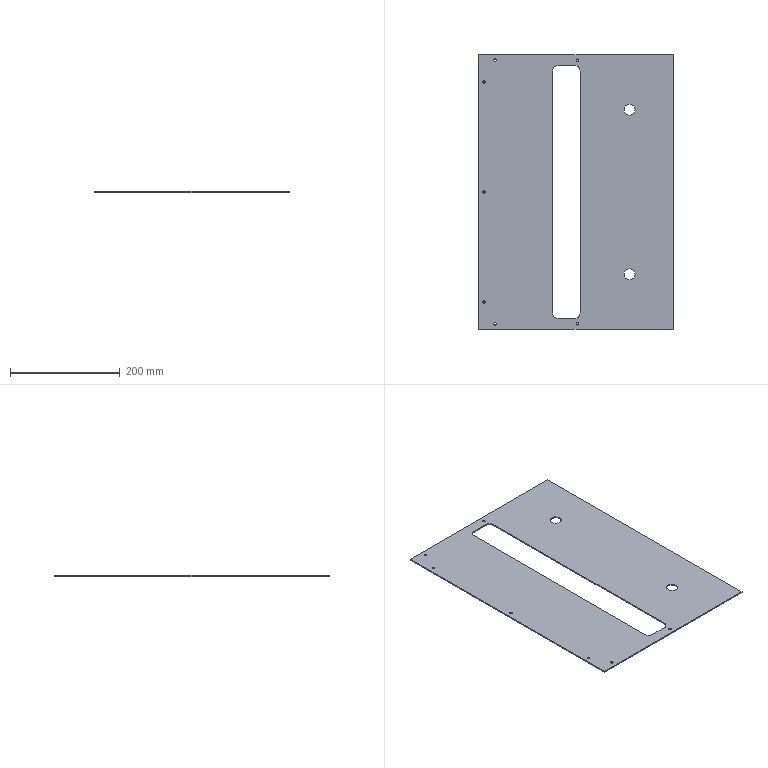Part | SolidWorks | features ICE 2, Extrusion 1, Fillet 1, HoleWzd 1 | 1 solid | 32 faces | box 355 x 500 x 2 mm | volume 307692 mm3 | cylinder 22 | plane 10 | commonest cylinder face diameters 4.5 x14 20 x8
STEP:
#1=CARTESIAN_POINT('',(87.5,150.,2.));
#2=VERTEX_POINT('',#1);
#3=CARTESIAN_POINT('',(107.5,150.,2.));
#4=VERTEX_POINT('',#3);
#5=CARTESIAN_POINT('',(97.5,150.,2.));
#6=DIRECTION('',(0.,0.,1.));
#7=DIRECTION('',(1.,0.,0.));
#8=AXIS2_PLACEMENT_3D('',#5,#6,#7);
#9=CIRCLE('',#8,10.);
#10=EDGE_CURVE('',#2,#4,#9,.T.);
#11=ORIENTED_EDGE('',*,*,#10,.T.);
#12=CARTESIAN_POINT('',(107.5,150.,0.));
#13=VERTEX_POINT('',#12);
#14=CARTESIAN_POINT('',(107.5,150.,10.));
#15=DIRECTION('',(0.,0.,-1.));
#16=VECTOR('',#15,1000.);
#17=LINE('',#14,#16);
#18=EDGE_CURVE('',#4,#13,#17,.T.);
#19=ORIENTED_EDGE('',*,*,#18,.T.);
#20=CARTESIAN_POINT('',(87.5,150.,0.));
#21=VERTEX_POINT('',#20);
#22=CARTESIAN_POINT('',(97.5,150.,0.));
#23=DIRECTION('',(0.,0.,-1.));
#24=DIRECTION('',(-1.,0.,0.));
#25=AXIS2_PLACEMENT_3D('',#22,#23,#24);
#26=CIRCLE('',#25,10.);
#27=EDGE_CURVE('',#13,#21,#26,.T.);
#28=ORIENTED_EDGE('',*,*,#27,.T.);
#29=CARTESIAN_POINT('',(87.5,150.,10.));
#30=DIRECTION('',(0.,0.,-1.));
#31=VECTOR('',#30,1000.);
#32=LINE('',#29,#31);
#33=EDGE_CURVE('',#2,#21,#32,.T.);
#34=ORIENTED_EDGE('',*,*,#33,.F.);
#35=EDGE_LOOP('',(#11,#19,#28,#34));
#36=FACE_OUTER_BOUND('',#35,.T.);
#37=CARTESIAN_POINT('',(97.5,150.,10.));
#38=DIRECTION('',(0.,0.,-1.));
#39=DIRECTION('',(-1.,0.,0.));
#40=AXIS2_PLACEMENT_3D('',#37,#38,#39);
#41=CYLINDRICAL_SURFACE('',#40,10.);
#42=ADVANCED_FACE('',(#36),#41,.F.);
#43=CARTESIAN_POINT('',(87.5,-150.,2.));
#44=VERTEX_POINT('',#43);
#45=CARTESIAN_POINT('',(107.5,-150.,2.));
#46=VERTEX_POINT('',#45);
#47=CARTESIAN_POINT('',(97.5,-150.,2.));
#48=DIRECTION('',(0.,0.,1.));
#49=DIRECTION('',(1.,0.,0.));
#50=AXIS2_PLACEMENT_3D('',#47,#48,#49);
#51=CIRCLE('',#50,10.);
#52=EDGE_CURVE('',#44,#46,#51,.T.);
#53=ORIENTED_EDGE('',*,*,#52,.T.);
#54=CARTESIAN_POINT('',(107.5,-150.,0.));
#55=VERTEX_POINT('',#54);
#56=CARTESIAN_POINT('',(107.5,-150.,10.));
#57=DIRECTION('',(0.,0.,-1.));
#58=VECTOR('',#57,1000.);
#59=LINE('',#56,#58);
#60=EDGE_CURVE('',#46,#55,#59,.T.);
#61=ORIENTED_EDGE('',*,*,#60,.T.);
#62=CARTESIAN_POINT('',(87.5,-150.,0.));
#63=VERTEX_POINT('',#62);
#64=CARTESIAN_POINT('',(97.5,-150.,0.));
#65=DIRECTION('',(0.,0.,-1.));
#66=DIRECTION('',(-1.,0.,0.));
#67=AXIS2_PLACEMENT_3D('',#64,#65,#66);
#68=CIRCLE('',#67,10.);
#69=EDGE_CURVE('',#55,#63,#68,.T.);
#70=ORIENTED_EDGE('',*,*,#69,.T.);
#71=CARTESIAN_POINT('',(87.5,-150.,10.));
#72=DIRECTION('',(0.,0.,-1.));
#73=VECTOR('',#72,1000.);
#74=LINE('',#71,#73);
#75=EDGE_CURVE('',#44,#63,#74,.T.);
#76=ORIENTED_EDGE('',*,*,#75,.F.);
#77=EDGE_LOOP('',(#53,#61,#70,#76));
#78=FACE_OUTER_BOUND('',#77,.T.);
#79=CARTESIAN_POINT('',(97.5,-150.,10.));
#80=DIRECTION('',(0.,0.,-1.));
#81=DIRECTION('',(-1.,0.,0.));
#82=AXIS2_PLACEMENT_3D('',#79,#80,#81);
#83=CYLINDRICAL_SURFACE('',#82,10.);
#84=ADVANCED_FACE('',(#78),#83,.F.);
#85=CARTESIAN_POINT('',(-169.75,0.,0.));
#86=VERTEX_POINT('',#85);
#87=CARTESIAN_POINT('',(-165.25,0.,0.));
#88=VERTEX_POINT('',#87);
#89=CARTESIAN_POINT('',(-167.5,0.,0.));
#90=DIRECTION('',(0.,0.,1.));
#91=DIRECTION('',(1.,0.,0.));
#92=AXIS2_PLACEMENT_3D('',#89,#90,#91);
#93=CIRCLE('',#92,2.25);
#94=EDGE_CURVE('',#86,#88,#93,.T.);
#95=ORIENTED_EDGE('',*,*,#94,.F.);
#96=CARTESIAN_POINT('',(-169.75,0.,2.));
#97=VERTEX_POINT('',#96);
#98=CARTESIAN_POINT('',(-169.75,0.,2.));
#99=DIRECTION('',(0.,0.,1.));
#100=VECTOR('',#99,1000.);
#101=LINE('',#98,#100);
#102=EDGE_CURVE('',#86,#97,#101,.T.);
#103=ORIENTED_EDGE('',*,*,#102,.T.);
#104=CARTESIAN_POINT('',(-165.25,0.,2.));
#105=VERTEX_POINT('',#104);
#106=CARTESIAN_POINT('',(-167.5,0.,2.));
#107=DIRECTION('',(0.,0.,1.));
#108=DIRECTION('',(1.,0.,0.));
#109=AXIS2_PLACEMENT_3D('',#106,#107,#108);
#110=CIRCLE('',#109,2.25);
#111=EDGE_CURVE('',#97,#105,#110,.T.);
#112=ORIENTED_EDGE('',*,*,#111,.T.);
#113=CARTESIAN_POINT('',(-165.25,0.,2.));
#114=DIRECTION('',(0.,0.,1.));
#115=VECTOR('',#114,1000.);
#116=LINE('',#113,#115);
#117=EDGE_CURVE('',#88,#105,#116,.T.);
#118=ORIENTED_EDGE('',*,*,#117,.F.);
#119=EDGE_LOOP('',(#95,#103,#112,#118));
#120=FACE_OUTER_BOUND('',#119,.T.);
#121=CARTESIAN_POINT('',(-167.5,0.,2.));
#122=DIRECTION('',(0.,0.,1.));
#123=DIRECTION('',(1.,0.,0.));
#124=AXIS2_PLACEMENT_3D('',#121,#122,#123);
#125=CYLINDRICAL_SURFACE('',#124,2.25);
#126=ADVANCED_FACE('',(#120),#125,.F.);
#127=CARTESIAN_POINT('',(-169.75,200.,0.));
#128=VERTEX_POINT('',#127);
#129=CARTESIAN_POINT('',(-165.25,200.,0.));
#130=VERTEX_POINT('',#129);
#131=CARTESIAN_POINT('',(-167.5,200.,0.));
#132=DIRECTION('',(0.,0.,1.));
#133=DIRECTION('',(1.,0.,0.));
#134=AXIS2_PLACEMENT_3D('',#131,#132,#133);
#135=CIRCLE('',#134,2.25);
#136=EDGE_CURVE('',#128,#130,#135,.T.);
#137=ORIENTED_EDGE('',*,*,#136,.F.);
#138=CARTESIAN_POINT('',(-169.75,200.,2.));
#139=VERTEX_POINT('',#138);
#140=CARTESIAN_POINT('',(-169.75,200.,2.));
#141=DIRECTION('',(0.,0.,1.));
#142=VECTOR('',#141,1000.);
#143=LINE('',#140,#142);
#144=EDGE_CURVE('',#128,#139,#143,.T.);
#145=ORIENTED_EDGE('',*,*,#144,.T.);
#146=CARTESIAN_POINT('',(-165.25,200.,2.));
#147=VERTEX_POINT('',#146);
#148=CARTESIAN_POINT('',(-167.5,200.,2.));
#149=DIRECTION('',(0.,0.,1.));
#150=DIRECTION('',(1.,0.,0.));
#151=AXIS2_PLACEMENT_3D('',#148,#149,#150);
#152=CIRCLE('',#151,2.25);
#153=EDGE_CURVE('',#139,#147,#152,.T.);
#154=ORIENTED_EDGE('',*,*,#153,.T.);
#155=CARTESIAN_POINT('',(-165.25,200.,2.));
#156=DIRECTION('',(0.,0.,1.));
#157=VECTOR('',#156,1000.);
#158=LINE('',#155,#157);
#159=EDGE_CURVE('',#130,#147,#158,.T.);
#160=ORIENTED_EDGE('',*,*,#159,.F.);
#161=EDGE_LOOP('',(#137,#145,#154,#160));
#162=FACE_OUTER_BOUND('',#161,.T.);
#163=CARTESIAN_POINT('',(-167.5,200.,2.));
#164=DIRECTION('',(0.,0.,1.));
#165=DIRECTION('',(1.,0.,0.));
#166=AXIS2_PLACEMENT_3D('',#163,#164,#165);
#167=CYLINDRICAL_SURFACE('',#166,2.25);
#168=ADVANCED_FACE('',(#162),#167,.F.);
#169=CARTESIAN_POINT('',(-169.75,-200.,0.));
#170=VERTEX_POINT('',#169);
#171=CARTESIAN_POINT('',(-165.25,-200.,0.));
#172=VERTEX_POINT('',#171);
#173=CARTESIAN_POINT('',(-167.5,-200.,0.));
#174=DIRECTION('',(0.,0.,1.));
#175=DIRECTION('',(1.,0.,0.));
#176=AXIS2_PLACEMENT_3D('',#173,#174,#175);
#177=CIRCLE('',#176,2.25);
#178=EDGE_CURVE('',#170,#172,#177,.T.);
#179=ORIENTED_EDGE('',*,*,#178,.F.);
#180=CARTESIAN_POINT('',(-169.75,-200.,2.));
#181=VERTEX_POINT('',#180);
#182=CARTESIAN_POINT('',(-169.75,-200.,2.));
#183=DIRECTION('',(0.,0.,1.));
#184=VECTOR('',#183,1000.);
#185=LINE('',#182,#184);
#186=EDGE_CURVE('',#170,#181,#185,.T.);
#187=ORIENTED_EDGE('',*,*,#186,.T.);
#188=CARTESIAN_POINT('',(-165.25,-200.,2.));
#189=VERTEX_POINT('',#188);
#190=CARTESIAN_POINT('',(-167.5,-200.,2.));
#191=DIRECTION('',(0.,0.,1.));
#192=DIRECTION('',(1.,0.,0.));
#193=AXIS2_PLACEMENT_3D('',#190,#191,#192);
#194=CIRCLE('',#193,2.25);
#195=EDGE_CURVE('',#181,#189,#194,.T.);
#196=ORIENTED_EDGE('',*,*,#195,.T.);
#197=CARTESIAN_POINT('',(-165.25,-200.,2.));
#198=DIRECTION('',(0.,0.,1.));
#199=VECTOR('',#198,1000.);
#200=LINE('',#197,#199);
#201=EDGE_CURVE('',#172,#189,#200,.T.);
#202=ORIENTED_EDGE('',*,*,#201,.F.);
#203=EDGE_LOOP('',(#179,#187,#196,#202));
#204=FACE_OUTER_BOUND('',#203,.T.);
#205=CARTESIAN_POINT('',(-167.5,-200.,2.));
#206=DIRECTION('',(0.,0.,1.));
#207=DIRECTION('',(1.,0.,0.));
#208=AXIS2_PLACEMENT_3D('',#205,#206,#207);
#209=CYLINDRICAL_SURFACE('',#208,2.25);
#210=ADVANCED_FACE('',(#204),#209,.F.);
#211=CARTESIAN_POINT('',(-149.75,240.,0.));
#212=VERTEX_POINT('',#211);
#213=CARTESIAN_POINT('',(-145.25,240.,0.));
#214=VERTEX_POINT('',#213);
#215=CARTESIAN_POINT('',(-147.5,240.,0.));
#216=DIRECTION('',(0.,0.,1.));
#217=DIRECTION('',(1.,0.,0.));
#218=AXIS2_PLACEMENT_3D('',#215,#216,#217);
#219=CIRCLE('',#218,2.25);
#220=EDGE_CURVE('',#212,#214,#219,.T.);
#221=ORIENTED_EDGE('',*,*,#220,.F.);
#222=CARTESIAN_POINT('',(-149.75,240.,2.));
#223=VERTEX_POINT('',#222);
#224=CARTESIAN_POINT('',(-149.75,240.,2.));
#225=DIRECTION('',(0.,0.,1.));
#226=VECTOR('',#225,1000.);
#227=LINE('',#224,#226);
#228=EDGE_CURVE('',#212,#223,#227,.T.);
#229=ORIENTED_EDGE('',*,*,#228,.T.);
#230=CARTESIAN_POINT('',(-145.25,240.,2.));
#231=VERTEX_POINT('',#230);
#232=CARTESIAN_POINT('',(-147.5,240.,2.));
#233=DIRECTION('',(0.,0.,1.));
#234=DIRECTION('',(1.,0.,0.));
#235=AXIS2_PLACEMENT_3D('',#232,#233,#234);
#236=CIRCLE('',#235,2.25);
#237=EDGE_CURVE('',#223,#231,#236,.T.);
#238=ORIENTED_EDGE('',*,*,#237,.T.);
#239=CARTESIAN_POINT('',(-145.25,240.,2.));
#240=DIRECTION('',(0.,0.,1.));
#241=VECTOR('',#240,1000.);
#242=LINE('',#239,#241);
#243=EDGE_CURVE('',#214,#231,#242,.T.);
#244=ORIENTED_EDGE('',*,*,#243,.F.);
#245=EDGE_LOOP('',(#221,#229,#238,#244));
#246=FACE_OUTER_BOUND('',#245,.T.);
#247=CARTESIAN_POINT('',(-147.5,240.,2.));
#248=DIRECTION('',(0.,0.,1.));
#249=DIRECTION('',(1.,0.,0.));
#250=AXIS2_PLACEMENT_3D('',#247,#248,#249);
#251=CYLINDRICAL_SURFACE('',#250,2.25);
#252=ADVANCED_FACE('',(#246),#251,.F.);
#253=CARTESIAN_POINT('',(0.25,240.,0.));
#254=VERTEX_POINT('',#253);
#255=CARTESIAN_POINT('',(4.75,240.,0.));
#256=VERTEX_POINT('',#255);
#257=CARTESIAN_POINT('',(2.5,240.,0.));
#258=DIRECTION('',(0.,0.,1.));
#259=DIRECTION('',(1.,0.,0.));
#260=AXIS2_PLACEMENT_3D('',#257,#258,#259);
#261=CIRCLE('',#260,2.25);
#262=EDGE_CURVE('',#254,#256,#261,.T.);
#263=ORIENTED_EDGE('',*,*,#262,.F.);
#264=CARTESIAN_POINT('',(0.25,240.,2.));
#265=VERTEX_POINT('',#264);
#266=CARTESIAN_POINT('',(0.25,240.,2.));
#267=DIRECTION('',(0.,0.,1.));
#268=VECTOR('',#267,1000.);
#269=LINE('',#266,#268);
#270=EDGE_CURVE('',#254,#265,#269,.T.);
#271=ORIENTED_EDGE('',*,*,#270,.T.);
#272=CARTESIAN_POINT('',(4.75,240.,2.));
#273=VERTEX_POINT('',#272);
#274=CARTESIAN_POINT('',(2.5,240.,2.));
#275=DIRECTION('',(0.,0.,1.));
#276=DIRECTION('',(1.,0.,0.));
#277=AXIS2_PLACEMENT_3D('',#274,#275,#276);
#278=CIRCLE('',#277,2.25);
#279=EDGE_CURVE('',#265,#273,#278,.T.);
#280=ORIENTED_EDGE('',*,*,#279,.T.);
#281=CARTESIAN_POINT('',(4.75,240.,2.));
#282=DIRECTION('',(0.,0.,1.));
#283=VECTOR('',#282,1000.);
#284=LINE('',#281,#283);
#285=EDGE_CURVE('',#256,#273,#284,.T.);
#286=ORIENTED_EDGE('',*,*,#285,.F.);
#287=EDGE_LOOP('',(#263,#271,#280,#286));
#288=FACE_OUTER_BOUND('',#287,.T.);
#289=CARTESIAN_POINT('',(2.5,240.,2.));
#290=DIRECTION('',(0.,0.,1.));
#291=DIRECTION('',(1.,0.,0.));
#292=AXIS2_PLACEMENT_3D('',#289,#290,#291);
#293=CYLINDRICAL_SURFACE('',#292,2.25);
#294=ADVANCED_FACE('',(#288),#293,.F.);
#295=CARTESIAN_POINT('',(0.25,-240.,0.));
#296=VERTEX_POINT('',#295);
#297=CARTESIAN_POINT('',(4.75,-240.,0.));
#298=VERTEX_POINT('',#297);
#299=CARTESIAN_POINT('',(2.5,-240.,0.));
#300=DIRECTION('',(0.,0.,1.));
#301=DIRECTION('',(1.,0.,0.));
#302=AXIS2_PLACEMENT_3D('',#299,#300,#301);
#303=CIRCLE('',#302,2.25);
#304=EDGE_CURVE('',#296,#298,#303,.T.);
#305=ORIENTED_EDGE('',*,*,#304,.F.);
#306=CARTESIAN_POINT('',(0.25,-240.,2.));
#307=VERTEX_POINT('',#306);
#308=CARTESIAN_POINT('',(0.25,-240.,2.));
#309=DIRECTION('',(0.,0.,1.));
#310=VECTOR('',#309,1000.);
#311=LINE('',#308,#310);
#312=EDGE_CURVE('',#296,#307,#311,.T.);
#313=ORIENTED_EDGE('',*,*,#312,.T.);
#314=CARTESIAN_POINT('',(4.75,-240.,2.));
#315=VERTEX_POINT('',#314);
#316=CARTESIAN_POINT('',(2.5,-240.,2.));
#317=DIRECTION('',(0.,0.,1.));
#318=DIRECTION('',(1.,0.,0.));
#319=AXIS2_PLACEMENT_3D('',#316,#317,#318);
#320=CIRCLE('',#319,2.25);
#321=EDGE_CURVE('',#307,#315,#320,.T.);
#322=ORIENTED_EDGE('',*,*,#321,.T.);
#323=CARTESIAN_POINT('',(4.75,-240.,2.));
#324=DIRECTION('',(0.,0.,1.));
#325=VECTOR('',#324,1000.);
#326=LINE('',#323,#325);
#327=EDGE_CURVE('',#298,#315,#326,.T.);
#328=ORIENTED_EDGE('',*,*,#327,.F.);
#329=EDGE_LOOP('',(#305,#313,#322,#328));
#330=FACE_OUTER_BOUND('',#329,.T.);
#331=CARTESIAN_POINT('',(2.5,-240.,2.));
#332=DIRECTION('',(0.,0.,1.));
#333=DIRECTION('',(1.,0.,0.));
#334=AXIS2_PLACEMENT_3D('',#331,#332,#333);
#335=CYLINDRICAL_SURFACE('',#334,2.25);
#336=ADVANCED_FACE('',(#330),#335,.F.);
#337=CARTESIAN_POINT('',(-149.75,-240.,0.));
#338=VERTEX_POINT('',#337);
#339=CARTESIAN_POINT('',(-145.25,-240.,0.));
#340=VERTEX_POINT('',#339);
#341=CARTESIAN_POINT('',(-147.5,-240.,0.));
#342=DIRECTION('',(0.,0.,1.));
#343=DIRECTION('',(1.,0.,0.));
#344=AXIS2_PLACEMENT_3D('',#341,#342,#343);
#345=CIRCLE('',#344,2.25);
#346=EDGE_CURVE('',#338,#340,#345,.T.);
#347=ORIENTED_EDGE('',*,*,#346,.F.);
#348=CARTESIAN_POINT('',(-149.75,-240.,2.));
#349=VERTEX_POINT('',#348);
#350=CARTESIAN_POINT('',(-149.75,-240.,2.));
#351=DIRECTION('',(0.,0.,1.));
#352=VECTOR('',#351,1000.);
#353=LINE('',#350,#352);
#354=EDGE_CURVE('',#338,#349,#353,.T.);
#355=ORIENTED_EDGE('',*,*,#354,.T.);
#356=CARTESIAN_POINT('',(-145.25,-240.,2.));
#357=VERTEX_POINT('',#356);
#358=CARTESIAN_POINT('',(-147.5,-240.,2.));
#359=DIRECTION('',(0.,0.,1.));
#360=DIRECTION('',(1.,0.,0.));
#361=AXIS2_PLACEMENT_3D('',#358,#359,#360);
#362=CIRCLE('',#361,2.25);
#363=EDGE_CURVE('',#349,#357,#362,.T.);
#364=ORIENTED_EDGE('',*,*,#363,.T.);
#365=CARTESIAN_POINT('',(-145.25,-240.,2.));
#366=DIRECTION('',(0.,0.,1.));
#367=VECTOR('',#366,1000.);
#368=LINE('',#365,#367);
#369=EDGE_CURVE('',#340,#357,#368,.T.);
#370=ORIENTED_EDGE('',*,*,#369,.F.);
#371=EDGE_LOOP('',(#347,#355,#364,#370));
#372=FACE_OUTER_BOUND('',#371,.T.);
#373=CARTESIAN_POINT('',(-147.5,-240.,2.));
#374=DIRECTION('',(0.,0.,1.));
#375=DIRECTION('',(1.,0.,0.));
#376=AXIS2_PLACEMENT_3D('',#373,#374,#375);
#377=CYLINDRICAL_SURFACE('',#376,2.25);
#378=ADVANCED_FACE('',(#372),#377,.F.);
#379=CARTESIAN_POINT('',(177.5,-250.,0.));
#380=VERTEX_POINT('',#379);
#381=CARTESIAN_POINT('',(177.5,250.,0.));
#382=VERTEX_POINT('',#381);
#383=CARTESIAN_POINT('',(177.5,250.,0.));
#384=DIRECTION('',(0.,1.,0.));
#385=VECTOR('',#384,1000.);
#386=LINE('',#383,#385);
#387=EDGE_CURVE('',#380,#382,#386,.T.);
#388=ORIENTED_EDGE('',*,*,#387,.T.);
#389=CARTESIAN_POINT('',(177.5,250.,2.));
#390=VERTEX_POINT('',#389);
#391=CARTESIAN_POINT('',(177.5,250.,2.));
#392=DIRECTION('',(0.,0.,-1.));
#393=VECTOR('',#392,1000.);
#394=LINE('',#391,#393);
#395=EDGE_CURVE('',#390,#382,#394,.T.);
#396=ORIENTED_EDGE('',*,*,#395,.F.);
#397=CARTESIAN_POINT('',(177.5,-250.,2.));
#398=VERTEX_POINT('',#397);
#399=CARTESIAN_POINT('',(177.5,250.,2.));
#400=DIRECTION('',(0.,1.,0.));
#401=VECTOR('',#400,1000.);
#402=LINE('',#399,#401);
#403=EDGE_CURVE('',#398,#390,#402,.T.);
#404=ORIENTED_EDGE('',*,*,#403,.F.);
#405=CARTESIAN_POINT('',(177.5,-250.,2.));
#406=DIRECTION('',(0.,0.,-1.));
#407=VECTOR('',#406,1000.);
#408=LINE('',#405,#407);
#409=EDGE_CURVE('',#398,#380,#408,.T.);
#410=ORIENTED_EDGE('',*,*,#409,.T.);
#411=EDGE_LOOP('',(#388,#396,#404,#410));
#412=FACE_OUTER_BOUND('',#411,.T.);
#413=CARTESIAN_POINT('',(177.5,250.,2.));
#414=DIRECTION('',(-1.,0.,0.));
#415=DIRECTION('',(0.,0.,1.));
#416=AXIS2_PLACEMENT_3D('',#413,#414,#415);
#417=PLANE('',#416);
#418=ADVANCED_FACE('',(#412),#417,.F.);
#419=CARTESIAN_POINT('',(-177.5,250.,0.));
#420=VERTEX_POINT('',#419);
#421=CARTESIAN_POINT('',(-177.5,250.,0.));
#422=DIRECTION('',(-1.,0.,0.));
#423=VECTOR('',#422,1000.);
#424=LINE('',#421,#423);
#425=EDGE_CURVE('',#382,#420,#424,.T.);
#426=ORIENTED_EDGE('',*,*,#425,.T.);
#427=CARTESIAN_POINT('',(-177.5,250.,2.));
#428=VERTEX_POINT('',#427);
#429=CARTESIAN_POINT('',(-177.5,250.,2.));
#430=DIRECTION('',(0.,0.,-1.));
#431=VECTOR('',#430,1000.);
#432=LINE('',#429,#431);
#433=EDGE_CURVE('',#428,#420,#432,.T.);
#434=ORIENTED_EDGE('',*,*,#433,.F.);
#435=CARTESIAN_POINT('',(-177.5,250.,2.));
#436=DIRECTION('',(-1.,0.,0.));
#437=VECTOR('',#436,1000.);
#438=LINE('',#435,#437);
#439=EDGE_CURVE('',#390,#428,#438,.T.);
#440=ORIENTED_EDGE('',*,*,#439,.F.);
#441=ORIENTED_EDGE('',*,*,#395,.T.);
#442=EDGE_LOOP('',(#426,#434,#440,#441));
#443=FACE_OUTER_BOUND('',#442,.T.);
#444=CARTESIAN_POINT('',(-177.5,250.,2.));
#445=DIRECTION('',(0.,-1.,0.));
#446=DIRECTION('',(0.,0.,-1.));
#447=AXIS2_PLACEMENT_3D('',#444,#445,#446);
#448=PLANE('',#447);
#449=ADVANCED_FACE('',(#443),#448,.F.);
#450=CARTESIAN_POINT('',(-177.5,-250.,0.));
#451=VERTEX_POINT('',#450);
#452=CARTESIAN_POINT('',(-177.5,250.,0.));
#453=DIRECTION('',(0.,-1.,0.));
#454=VECTOR('',#453,1000.);
#455=LINE('',#452,#454);
#456=EDGE_CURVE('',#420,#451,#455,.T.);
#457=ORIENTED_EDGE('',*,*,#456,.T.);
#458=CARTESIAN_POINT('',(-177.5,-250.,2.));
#459=VERTEX_POINT('',#458);
#460=CARTESIAN_POINT('',(-177.5,-250.,2.));
#461=DIRECTION('',(0.,0.,-1.));
#462=VECTOR('',#461,1000.);
#463=LINE('',#460,#462);
#464=EDGE_CURVE('',#459,#451,#463,.T.);
#465=ORIENTED_EDGE('',*,*,#464,.F.);
#466=CARTESIAN_POINT('',(-177.5,250.,2.));
#467=DIRECTION('',(0.,-1.,0.));
#468=VECTOR('',#467,1000.);
#469=LINE('',#466,#468);
#470=EDGE_CURVE('',#428,#459,#469,.T.);
#471=ORIENTED_EDGE('',*,*,#470,.F.);
#472=ORIENTED_EDGE('',*,*,#433,.T.);
#473=EDGE_LOOP('',(#457,#465,#471,#472));
#474=FACE_OUTER_BOUND('',#473,.T.);
#475=CARTESIAN_POINT('',(-177.5,250.,2.));
#476=DIRECTION('',(1.,0.,0.));
#477=DIRECTION('',(0.,0.,-1.));
#478=AXIS2_PLACEMENT_3D('',#475,#476,#477);
#479=PLANE('',#478);
#480=ADVANCED_FACE('',(#474),#479,.F.);
#481=CARTESIAN_POINT('',(-177.5,-250.,0.));
#482=DIRECTION('',(1.,0.,0.));
#483=VECTOR('',#482,1000.);
#484=LINE('',#481,#483);
#485=EDGE_CURVE('',#451,#380,#484,.T.);
#486=ORIENTED_EDGE('',*,*,#485,.T.);
#487=ORIENTED_EDGE('',*,*,#409,.F.);
#488=CARTESIAN_POINT('',(-177.5,-250.,2.));
#489=DIRECTION('',(1.,0.,0.));
#490=VECTOR('',#489,1000.);
#491=LINE('',#488,#490);
#492=EDGE_CURVE('',#459,#398,#491,.T.);
#493=ORIENTED_EDGE('',*,*,#492,.F.);
#494=ORIENTED_EDGE('',*,*,#464,.T.);
#495=EDGE_LOOP('',(#486,#487,#493,#494));
#496=FACE_OUTER_BOUND('',#495,.T.);
#497=CARTESIAN_POINT('',(-177.5,-250.,2.));
#498=DIRECTION('',(0.,1.,0.));
#499=DIRECTION('',(0.,0.,1.));
#500=AXIS2_PLACEMENT_3D('',#497,#498,#499);
#501=PLANE('',#500);
#502=ADVANCED_FACE('',(#496),#501,.F.);
#503=ORIENTED_EDGE('',*,*,#10,.F.);
#504=CARTESIAN_POINT('',(97.5,150.,2.));
#505=DIRECTION('',(0.,0.,1.));
#506=DIRECTION('',(1.,0.,0.));
#507=AXIS2_PLACEMENT_3D('',#504,#505,#506);
#508=CIRCLE('',#507,10.);
#509=EDGE_CURVE('',#4,#2,#508,.T.);
#510=ORIENTED_EDGE('',*,*,#509,.F.);
#511=EDGE_LOOP('',(#503,#510));
#512=FACE_BOUND('',#511,.T.);
#513=ORIENTED_EDGE('',*,*,#52,.F.);
#514=CARTESIAN_POINT('',(97.5,-150.,2.));
#515=DIRECTION('',(0.,0.,1.));
#516=DIRECTION('',(1.,0.,0.));
#517=AXIS2_PLACEMENT_3D('',#514,#515,#516);
#518=CIRCLE('',#517,10.);
#519=EDGE_CURVE('',#46,#44,#518,.T.);
#520=ORIENTED_EDGE('',*,*,#519,.F.);
#521=EDGE_LOOP('',(#513,#520));
#522=FACE_BOUND('',#521,.T.);
#523=CARTESIAN_POINT('',(-42.5,220.,2.));
#524=VERTEX_POINT('',#523);
#525=CARTESIAN_POINT('',(-42.5,-220.,2.));
#526=VERTEX_POINT('',#525);
#527=CARTESIAN_POINT('',(-42.5,0.,2.));
#528=DIRECTION('',(0.,-1.,0.));
#529=VECTOR('',#528,1000.);
#530=LINE('',#527,#529);
#531=EDGE_CURVE('',#524,#526,#530,.T.);
#532=ORIENTED_EDGE('',*,*,#531,.F.);
#533=CARTESIAN_POINT('',(-32.5,230.,2.));
#534=VERTEX_POINT('',#533);
#535=CARTESIAN_POINT('',(-32.5,220.,2.));
#536=DIRECTION('',(0.,0.,-1.));
#537=DIRECTION('',(1.,0.,0.));
#538=AXIS2_PLACEMENT_3D('',#535,#536,#537);
#539=CIRCLE('',#538,10.);
#540=EDGE_CURVE('',#524,#534,#539,.T.);
#541=ORIENTED_EDGE('',*,*,#540,.T.);
#542=CARTESIAN_POINT('',(-2.5,230.,2.));
#543=VERTEX_POINT('',#542);
#544=CARTESIAN_POINT('',(0.,230.,2.));
#545=DIRECTION('',(-1.,0.,0.));
#546=VECTOR('',#545,1000.);
#547=LINE('',#544,#546);
#548=EDGE_CURVE('',#543,#534,#547,.T.);
#549=ORIENTED_EDGE('',*,*,#548,.F.);
#550=CARTESIAN_POINT('',(7.5,220.,2.));
#551=VERTEX_POINT('',#550);
#552=CARTESIAN_POINT('',(-2.5,220.,2.));
#553=DIRECTION('',(0.,0.,-1.));
#554=DIRECTION('',(1.,0.,0.));
#555=AXIS2_PLACEMENT_3D('',#552,#553,#554);
#556=CIRCLE('',#555,10.);
#557=EDGE_CURVE('',#543,#551,#556,.T.);
#558=ORIENTED_EDGE('',*,*,#557,.T.);
#559=CARTESIAN_POINT('',(7.5,-220.,2.));
#560=VERTEX_POINT('',#559);
#561=CARTESIAN_POINT('',(7.5,0.,2.));
#562=DIRECTION('',(0.,1.,0.));
#563=VECTOR('',#562,1000.);
#564=LINE('',#561,#563);
#565=EDGE_CURVE('',#560,#551,#564,.T.);
#566=ORIENTED_EDGE('',*,*,#565,.F.);
#567=CARTESIAN_POINT('',(-2.5,-230.,2.));
#568=VERTEX_POINT('',#567);
#569=CARTESIAN_POINT('',(-2.5,-220.,2.));
#570=DIRECTION('',(0.,0.,-1.));
#571=DIRECTION('',(1.,0.,0.));
#572=AXIS2_PLACEMENT_3D('',#569,#570,#571);
#573=CIRCLE('',#572,10.);
#574=EDGE_CURVE('',#560,#568,#573,.T.);
#575=ORIENTED_EDGE('',*,*,#574,.T.);
#576=CARTESIAN_POINT('',(-32.5,-230.,2.));
#577=VERTEX_POINT('',#576);
#578=CARTESIAN_POINT('',(0.,-230.,2.));
#579=DIRECTION('',(1.,0.,0.));
#580=VECTOR('',#579,1000.);
#581=LINE('',#578,#580);
#582=EDGE_CURVE('',#577,#568,#581,.T.);
#583=ORIENTED_EDGE('',*,*,#582,.F.);
#584=CARTESIAN_POINT('',(-32.5,-220.,2.));
#585=DIRECTION('',(0.,0.,-1.));
#586=DIRECTION('',(1.,0.,0.));
#587=AXIS2_PLACEMENT_3D('',#584,#585,#586);
#588=CIRCLE('',#587,10.);
#589=EDGE_CURVE('',#577,#526,#588,.T.);
#590=ORIENTED_EDGE('',*,*,#589,.T.);
#591=EDGE_LOOP('',(#532,#541,#549,#558,#566,#575,#583,#590));
#592=FACE_BOUND('',#591,.T.);
#593=CARTESIAN_POINT('',(-167.5,0.,2.));
#594=DIRECTION('',(0.,0.,1.));
#595=DIRECTION('',(1.,0.,0.));
#596=AXIS2_PLACEMENT_3D('',#593,#594,#595);
#597=CIRCLE('',#596,2.25);
#598=EDGE_CURVE('',#105,#97,#597,.T.);
#599=ORIENTED_EDGE('',*,*,#598,.F.);
#600=ORIENTED_EDGE('',*,*,#111,.F.);
#601=EDGE_LOOP('',(#599,#600));
#602=FACE_BOUND('',#601,.T.);
#603=CARTESIAN_POINT('',(-167.5,200.,2.));
#604=DIRECTION('',(0.,0.,1.));
#605=DIRECTION('',(1.,0.,0.));
#606=AXIS2_PLACEMENT_3D('',#603,#604,#605);
#607=CIRCLE('',#606,2.25);
#608=EDGE_CURVE('',#147,#139,#607,.T.);
#609=ORIENTED_EDGE('',*,*,#608,.F.);
#610=ORIENTED_EDGE('',*,*,#153,.F.);
#611=EDGE_LOOP('',(#609,#610));
#612=FACE_BOUND('',#611,.T.);
#613=CARTESIAN_POINT('',(-167.5,-200.,2.));
#614=DIRECTION('',(0.,0.,1.));
#615=DIRECTION('',(1.,0.,0.));
#616=AXIS2_PLACEMENT_3D('',#613,#614,#615);
#617=CIRCLE('',#616,2.25);
#618=EDGE_CURVE('',#189,#181,#617,.T.);
#619=ORIENTED_EDGE('',*,*,#618,.F.);
#620=ORIENTED_EDGE('',*,*,#195,.F.);
#621=EDGE_LOOP('',(#619,#620));
#622=FACE_BOUND('',#621,.T.);
#623=CARTESIAN_POINT('',(-147.5,240.,2.));
#624=DIRECTION('',(0.,0.,1.));
#625=DIRECTION('',(1.,0.,0.));
#626=AXIS2_PLACEMENT_3D('',#623,#624,#625);
#627=CIRCLE('',#626,2.25);
#628=EDGE_CURVE('',#231,#223,#627,.T.);
#629=ORIENTED_EDGE('',*,*,#628,.F.);
#630=ORIENTED_EDGE('',*,*,#237,.F.);
#631=EDGE_LOOP('',(#629,#630));
#632=FACE_BOUND('',#631,.T.);
#633=CARTESIAN_POINT('',(2.5,240.,2.));
#634=DIRECTION('',(0.,0.,1.));
#635=DIRECTION('',(1.,0.,0.));
#636=AXIS2_PLACEMENT_3D('',#633,#634,#635);
#637=CIRCLE('',#636,2.25);
#638=EDGE_CURVE('',#273,#265,#637,.T.);
#639=ORIENTED_EDGE('',*,*,#638,.F.);
#640=ORIENTED_EDGE('',*,*,#279,.F.);
#641=EDGE_LOOP('',(#639,#640));
#642=FACE_BOUND('',#641,.T.);
#643=CARTESIAN_POINT('',(2.5,-240.,2.));
#644=DIRECTION('',(0.,0.,1.));
#645=DIRECTION('',(1.,0.,0.));
#646=AXIS2_PLACEMENT_3D('',#643,#644,#645);
#647=CIRCLE('',#646,2.25);
#648=EDGE_CURVE('',#315,#307,#647,.T.);
#649=ORIENTED_EDGE('',*,*,#648,.F.);
#650=ORIENTED_EDGE('',*,*,#321,.F.);
#651=EDGE_LOOP('',(#649,#650));
#652=FACE_BOUND('',#651,.T.);
#653=CARTESIAN_POINT('',(-147.5,-240.,2.));
#654=DIRECTION('',(0.,0.,1.));
#655=DIRECTION('',(1.,0.,0.));
#656=AXIS2_PLACEMENT_3D('',#653,#654,#655);
#657=CIRCLE('',#656,2.25);
#658=EDGE_CURVE('',#357,#349,#657,.T.);
#659=ORIENTED_EDGE('',*,*,#658,.F.);
#660=ORIENTED_EDGE('',*,*,#363,.F.);
#661=EDGE_LOOP('',(#659,#660));
#662=FACE_BOUND('',#661,.T.);
#663=ORIENTED_EDGE('',*,*,#403,.T.);
#664=ORIENTED_EDGE('',*,*,#439,.T.);
#665=ORIENTED_EDGE('',*,*,#470,.T.);
#666=ORIENTED_EDGE('',*,*,#492,.T.);
#667=EDGE_LOOP('',(#663,#664,#665,#666));
#668=FACE_OUTER_BOUND('',#667,.T.);
#669=CARTESIAN_POINT('',(0.,0.,2.));
#670=DIRECTION('',(0.,0.,1.));
#671=DIRECTION('',(1.,0.,0.));
#672=AXIS2_PLACEMENT_3D('',#669,#670,#671);
#673=PLANE('',#672);
#674=ADVANCED_FACE('',(#512,#522,#592,#602,#612,#622,#632,#642,#652,#662,#668),#673,.T.);
#675=CARTESIAN_POINT('',(97.5,150.,0.));
#676=DIRECTION('',(0.,0.,-1.));
#677=DIRECTION('',(-1.,0.,0.));
#678=AXIS2_PLACEMENT_3D('',#675,#676,#677);
#679=CIRCLE('',#678,10.);
#680=EDGE_CURVE('',#21,#13,#679,.T.);
#681=ORIENTED_EDGE('',*,*,#680,.F.);
#682=ORIENTED_EDGE('',*,*,#27,.F.);
#683=EDGE_LOOP('',(#681,#682));
#684=FACE_BOUND('',#683,.T.);
#685=CARTESIAN_POINT('',(97.5,-150.,0.));
#686=DIRECTION('',(0.,0.,-1.));
#687=DIRECTION('',(-1.,0.,0.));
#688=AXIS2_PLACEMENT_3D('',#685,#686,#687);
#689=CIRCLE('',#688,10.);
#690=EDGE_CURVE('',#63,#55,#689,.T.);
#691=ORIENTED_EDGE('',*,*,#690,.F.);
#692=ORIENTED_EDGE('',*,*,#69,.F.);
#693=EDGE_LOOP('',(#691,#692));
#694=FACE_BOUND('',#693,.T.);
#695=CARTESIAN_POINT('',(-32.5,230.,0.));
#696=VERTEX_POINT('',#695);
#697=CARTESIAN_POINT('',(-2.5,230.,0.));
#698=VERTEX_POINT('',#697);
#699=CARTESIAN_POINT('',(7.5,230.,0.));
#700=DIRECTION('',(1.,0.,0.));
#701=VECTOR('',#700,1000.);
#702=LINE('',#699,#701);
#703=EDGE_CURVE('',#696,#698,#702,.T.);
#704=ORIENTED_EDGE('',*,*,#703,.F.);
#705=CARTESIAN_POINT('',(-42.5,220.,0.));
#706=VERTEX_POINT('',#705);
#707=CARTESIAN_POINT('',(-32.5,220.,0.));
#708=DIRECTION('',(0.,0.,1.));
#709=DIRECTION('',(1.,0.,0.));
#710=AXIS2_PLACEMENT_3D('',#707,#708,#709);
#711=CIRCLE('',#710,10.);
#712=EDGE_CURVE('',#696,#706,#711,.T.);
#713=ORIENTED_EDGE('',*,*,#712,.T.);
#714=CARTESIAN_POINT('',(-42.5,-220.,0.));
#715=VERTEX_POINT('',#714);
#716=CARTESIAN_POINT('',(-42.5,-230.,0.));
#717=DIRECTION('',(0.,1.,0.));
#718=VECTOR('',#717,1000.);
#719=LINE('',#716,#718);
#720=EDGE_CURVE('',#715,#706,#719,.T.);
#721=ORIENTED_EDGE('',*,*,#720,.F.);
#722=CARTESIAN_POINT('',(-32.5,-230.,0.));
#723=VERTEX_POINT('',#722);
#724=CARTESIAN_POINT('',(-32.5,-220.,0.));
#725=DIRECTION('',(0.,0.,1.));
#726=DIRECTION('',(1.,0.,0.));
#727=AXIS2_PLACEMENT_3D('',#724,#725,#726);
#728=CIRCLE('',#727,10.);
#729=EDGE_CURVE('',#715,#723,#728,.T.);
#730=ORIENTED_EDGE('',*,*,#729,.T.);
#731=CARTESIAN_POINT('',(-2.5,-230.,0.));
#732=VERTEX_POINT('',#731);
#733=CARTESIAN_POINT('',(7.5,-230.,0.));
#734=DIRECTION('',(-1.,0.,0.));
#735=VECTOR('',#734,1000.);
#736=LINE('',#733,#735);
#737=EDGE_CURVE('',#732,#723,#736,.T.);
#738=ORIENTED_EDGE('',*,*,#737,.F.);
#739=CARTESIAN_POINT('',(7.5,-220.,0.));
#740=VERTEX_POINT('',#739);
#741=CARTESIAN_POINT('',(-2.5,-220.,0.));
#742=DIRECTION('',(0.,0.,1.));
#743=DIRECTION('',(1.,0.,0.));
#744=AXIS2_PLACEMENT_3D('',#741,#742,#743);
#745=CIRCLE('',#744,10.);
#746=EDGE_CURVE('',#732,#740,#745,.T.);
#747=ORIENTED_EDGE('',*,*,#746,.T.);
#748=CARTESIAN_POINT('',(7.5,220.,0.));
#749=VERTEX_POINT('',#748);
#750=CARTESIAN_POINT('',(7.5,-230.,0.));
#751=DIRECTION('',(0.,-1.,0.));
#752=VECTOR('',#751,1000.);
#753=LINE('',#750,#752);
#754=EDGE_CURVE('',#749,#740,#753,.T.);
#755=ORIENTED_EDGE('',*,*,#754,.F.);
#756=CARTESIAN_POINT('',(-2.5,220.,0.));
#757=DIRECTION('',(0.,0.,1.));
#758=DIRECTION('',(1.,0.,0.));
#759=AXIS2_PLACEMENT_3D('',#756,#757,#758);
#760=CIRCLE('',#759,10.);
#761=EDGE_CURVE('',#749,#698,#760,.T.);
#762=ORIENTED_EDGE('',*,*,#761,.T.);
#763=EDGE_LOOP('',(#704,#713,#721,#730,#738,#747,#755,#762));
#764=FACE_BOUND('',#763,.T.);
#765=CARTESIAN_POINT('',(-167.5,0.,0.));
#766=DIRECTION('',(0.,0.,1.));
#767=DIRECTION('',(1.,0.,0.));
#768=AXIS2_PLACEMENT_3D('',#765,#766,#767);
#769=CIRCLE('',#768,2.25);
#770=EDGE_CURVE('',#88,#86,#769,.T.);
#771=ORIENTED_EDGE('',*,*,#770,.T.);
#772=ORIENTED_EDGE('',*,*,#94,.T.);
#773=EDGE_LOOP('',(#771,#772));
#774=FACE_BOUND('',#773,.T.);
#775=CARTESIAN_POINT('',(-167.5,200.,0.));
#776=DIRECTION('',(0.,0.,1.));
#777=DIRECTION('',(1.,0.,0.));
#778=AXIS2_PLACEMENT_3D('',#775,#776,#777);
#779=CIRCLE('',#778,2.25);
#780=EDGE_CURVE('',#130,#128,#779,.T.);
#781=ORIENTED_EDGE('',*,*,#780,.T.);
#782=ORIENTED_EDGE('',*,*,#136,.T.);
#783=EDGE_LOOP('',(#781,#782));
#784=FACE_BOUND('',#783,.T.);
#785=CARTESIAN_POINT('',(-167.5,-200.,0.));
#786=DIRECTION('',(0.,0.,1.));
#787=DIRECTION('',(1.,0.,0.));
#788=AXIS2_PLACEMENT_3D('',#785,#786,#787);
#789=CIRCLE('',#788,2.25);
#790=EDGE_CURVE('',#172,#170,#789,.T.);
#791=ORIENTED_EDGE('',*,*,#790,.T.);
#792=ORIENTED_EDGE('',*,*,#178,.T.);
#793=EDGE_LOOP('',(#791,#792));
#794=FACE_BOUND('',#793,.T.);
#795=CARTESIAN_POINT('',(-147.5,240.,0.));
#796=DIRECTION('',(0.,0.,1.));
#797=DIRECTION('',(1.,0.,0.));
#798=AXIS2_PLACEMENT_3D('',#795,#796,#797);
#799=CIRCLE('',#798,2.25);
#800=EDGE_CURVE('',#214,#212,#799,.T.);
#801=ORIENTED_EDGE('',*,*,#800,.T.);
#802=ORIENTED_EDGE('',*,*,#220,.T.);
#803=EDGE_LOOP('',(#801,#802));
#804=FACE_BOUND('',#803,.T.);
#805=CARTESIAN_POINT('',(2.5,240.,0.));
#806=DIRECTION('',(0.,0.,1.));
#807=DIRECTION('',(1.,0.,0.));
#808=AXIS2_PLACEMENT_3D('',#805,#806,#807);
#809=CIRCLE('',#808,2.25);
#810=EDGE_CURVE('',#256,#254,#809,.T.);
#811=ORIENTED_EDGE('',*,*,#810,.T.);
#812=ORIENTED_EDGE('',*,*,#262,.T.);
#813=EDGE_LOOP('',(#811,#812));
#814=FACE_BOUND('',#813,.T.);
#815=CARTESIAN_POINT('',(2.5,-240.,0.));
#816=DIRECTION('',(0.,0.,1.));
#817=DIRECTION('',(1.,0.,0.));
#818=AXIS2_PLACEMENT_3D('',#815,#816,#817);
#819=CIRCLE('',#818,2.25);
#820=EDGE_CURVE('',#298,#296,#819,.T.);
#821=ORIENTED_EDGE('',*,*,#820,.T.);
#822=ORIENTED_EDGE('',*,*,#304,.T.);
#823=EDGE_LOOP('',(#821,#822));
#824=FACE_BOUND('',#823,.T.);
#825=CARTESIAN_POINT('',(-147.5,-240.,0.));
#826=DIRECTION('',(0.,0.,1.));
#827=DIRECTION('',(1.,0.,0.));
#828=AXIS2_PLACEMENT_3D('',#825,#826,#827);
#829=CIRCLE('',#828,2.25);
#830=EDGE_CURVE('',#340,#338,#829,.T.);
#831=ORIENTED_EDGE('',*,*,#830,.T.);
#832=ORIENTED_EDGE('',*,*,#346,.T.);
#833=EDGE_LOOP('',(#831,#832));
#834=FACE_BOUND('',#833,.T.);
#835=ORIENTED_EDGE('',*,*,#387,.F.);
#836=ORIENTED_EDGE('',*,*,#485,.F.);
#837=ORIENTED_EDGE('',*,*,#456,.F.);
#838=ORIENTED_EDGE('',*,*,#425,.F.);
#839=EDGE_LOOP('',(#835,#836,#837,#838));
#840=FACE_OUTER_BOUND('',#839,.T.);
#841=CARTESIAN_POINT('',(0.,0.,0.));
#842=DIRECTION('',(0.,0.,1.));
#843=DIRECTION('',(1.,0.,0.));
#844=AXIS2_PLACEMENT_3D('',#841,#842,#843);
#845=PLANE('',#844);
#846=ADVANCED_FACE('',(#684,#694,#764,#774,#784,#794,#804,#814,#824,#834,#840),#845,.F.);
#847=ORIENTED_EDGE('',*,*,#354,.F.);
#848=ORIENTED_EDGE('',*,*,#830,.F.);
#849=ORIENTED_EDGE('',*,*,#369,.T.);
#850=ORIENTED_EDGE('',*,*,#658,.T.);
#851=EDGE_LOOP('',(#847,#848,#849,#850));
#852=FACE_OUTER_BOUND('',#851,.T.);
#853=CARTESIAN_POINT('',(-147.5,-240.,2.));
#854=DIRECTION('',(0.,0.,1.));
#855=DIRECTION('',(1.,0.,0.));
#856=AXIS2_PLACEMENT_3D('',#853,#854,#855);
#857=CYLINDRICAL_SURFACE('',#856,2.25);
#858=ADVANCED_FACE('',(#852),#857,.F.);
#859=ORIENTED_EDGE('',*,*,#312,.F.);
#860=ORIENTED_EDGE('',*,*,#820,.F.);
#861=ORIENTED_EDGE('',*,*,#327,.T.);
#862=ORIENTED_EDGE('',*,*,#648,.T.);
#863=EDGE_LOOP('',(#859,#860,#861,#862));
#864=FACE_OUTER_BOUND('',#863,.T.);
#865=CARTESIAN_POINT('',(2.5,-240.,2.));
#866=DIRECTION('',(0.,0.,1.));
#867=DIRECTION('',(1.,0.,0.));
#868=AXIS2_PLACEMENT_3D('',#865,#866,#867);
#869=CYLINDRICAL_SURFACE('',#868,2.25);
#870=ADVANCED_FACE('',(#864),#869,.F.);
#871=ORIENTED_EDGE('',*,*,#270,.F.);
#872=ORIENTED_EDGE('',*,*,#810,.F.);
#873=ORIENTED_EDGE('',*,*,#285,.T.);
#874=ORIENTED_EDGE('',*,*,#638,.T.);
#875=EDGE_LOOP('',(#871,#872,#873,#874));
#876=FACE_OUTER_BOUND('',#875,.T.);
#877=CARTESIAN_POINT('',(2.5,240.,2.));
#878=DIRECTION('',(0.,0.,1.));
#879=DIRECTION('',(1.,0.,0.));
#880=AXIS2_PLACEMENT_3D('',#877,#878,#879);
#881=CYLINDRICAL_SURFACE('',#880,2.25);
#882=ADVANCED_FACE('',(#876),#881,.F.);
#883=ORIENTED_EDGE('',*,*,#228,.F.);
#884=ORIENTED_EDGE('',*,*,#800,.F.);
#885=ORIENTED_EDGE('',*,*,#243,.T.);
#886=ORIENTED_EDGE('',*,*,#628,.T.);
#887=EDGE_LOOP('',(#883,#884,#885,#886));
#888=FACE_OUTER_BOUND('',#887,.T.);
#889=CARTESIAN_POINT('',(-147.5,240.,2.));
#890=DIRECTION('',(0.,0.,1.));
#891=DIRECTION('',(1.,0.,0.));
#892=AXIS2_PLACEMENT_3D('',#889,#890,#891);
#893=CYLINDRICAL_SURFACE('',#892,2.25);
#894=ADVANCED_FACE('',(#888),#893,.F.);
#895=ORIENTED_EDGE('',*,*,#186,.F.);
#896=ORIENTED_EDGE('',*,*,#790,.F.);
#897=ORIENTED_EDGE('',*,*,#201,.T.);
#898=ORIENTED_EDGE('',*,*,#618,.T.);
#899=EDGE_LOOP('',(#895,#896,#897,#898));
#900=FACE_OUTER_BOUND('',#899,.T.);
#901=CARTESIAN_POINT('',(-167.5,-200.,2.));
#902=DIRECTION('',(0.,0.,1.));
#903=DIRECTION('',(1.,0.,0.));
#904=AXIS2_PLACEMENT_3D('',#901,#902,#903);
#905=CYLINDRICAL_SURFACE('',#904,2.25);
#906=ADVANCED_FACE('',(#900),#905,.F.);
#907=ORIENTED_EDGE('',*,*,#144,.F.);
#908=ORIENTED_EDGE('',*,*,#780,.F.);
#909=ORIENTED_EDGE('',*,*,#159,.T.);
#910=ORIENTED_EDGE('',*,*,#608,.T.);
#911=EDGE_LOOP('',(#907,#908,#909,#910));
#912=FACE_OUTER_BOUND('',#911,.T.);
#913=CARTESIAN_POINT('',(-167.5,200.,2.));
#914=DIRECTION('',(0.,0.,1.));
#915=DIRECTION('',(1.,0.,0.));
#916=AXIS2_PLACEMENT_3D('',#913,#914,#915);
#917=CYLINDRICAL_SURFACE('',#916,2.25);
#918=ADVANCED_FACE('',(#912),#917,.F.);
#919=ORIENTED_EDGE('',*,*,#102,.F.);
#920=ORIENTED_EDGE('',*,*,#770,.F.);
#921=ORIENTED_EDGE('',*,*,#117,.T.);
#922=ORIENTED_EDGE('',*,*,#598,.T.);
#923=EDGE_LOOP('',(#919,#920,#921,#922));
#924=FACE_OUTER_BOUND('',#923,.T.);
#925=CARTESIAN_POINT('',(-167.5,0.,2.));
#926=DIRECTION('',(0.,0.,1.));
#927=DIRECTION('',(1.,0.,0.));
#928=AXIS2_PLACEMENT_3D('',#925,#926,#927);
#929=CYLINDRICAL_SURFACE('',#928,2.25);
#930=ADVANCED_FACE('',(#924),#929,.F.);
#931=ORIENTED_EDGE('',*,*,#531,.T.);
#932=CARTESIAN_POINT('',(-42.5,-220.,0.));
#933=DIRECTION('',(0.,0.,-1.));
#934=VECTOR('',#933,1000.);
#935=LINE('',#932,#934);
#936=EDGE_CURVE('',#526,#715,#935,.T.);
#937=ORIENTED_EDGE('',*,*,#936,.T.);
#938=ORIENTED_EDGE('',*,*,#720,.T.);
#939=CARTESIAN_POINT('',(-42.5,220.,2.));
#940=DIRECTION('',(0.,0.,1.));
#941=VECTOR('',#940,1000.);
#942=LINE('',#939,#941);
#943=EDGE_CURVE('',#706,#524,#942,.T.);
#944=ORIENTED_EDGE('',*,*,#943,.T.);
#945=EDGE_LOOP('',(#931,#937,#938,#944));
#946=FACE_OUTER_BOUND('',#945,.T.);
#947=CARTESIAN_POINT('',(-42.5,-230.,10.));
#948=DIRECTION('',(-1.,0.,0.));
#949=DIRECTION('',(0.,0.,1.));
#950=AXIS2_PLACEMENT_3D('',#947,#948,#949);
#951=PLANE('',#950);
#952=ADVANCED_FACE('',(#946),#951,.F.);
#953=ORIENTED_EDGE('',*,*,#737,.T.);
#954=CARTESIAN_POINT('',(-32.5,-230.,2.));
#955=DIRECTION('',(0.,0.,1.));
#956=VECTOR('',#955,1000.);
#957=LINE('',#954,#956);
#958=EDGE_CURVE('',#723,#577,#957,.T.);
#959=ORIENTED_EDGE('',*,*,#958,.T.);
#960=ORIENTED_EDGE('',*,*,#582,.T.);
#961=CARTESIAN_POINT('',(-2.5,-230.,0.));
#962=DIRECTION('',(0.,0.,-1.));
#963=VECTOR('',#962,1000.);
#964=LINE('',#961,#963);
#965=EDGE_CURVE('',#568,#732,#964,.T.);
#966=ORIENTED_EDGE('',*,*,#965,.T.);
#967=EDGE_LOOP('',(#953,#959,#960,#966));
#968=FACE_OUTER_BOUND('',#967,.T.);
#969=CARTESIAN_POINT('',(7.5,-230.,10.));
#970=DIRECTION('',(0.,-1.,0.));
#971=DIRECTION('',(0.,0.,-1.));
#972=AXIS2_PLACEMENT_3D('',#969,#970,#971);
#973=PLANE('',#972);
#974=ADVANCED_FACE('',(#968),#973,.F.);
#975=ORIENTED_EDGE('',*,*,#754,.T.);
#976=CARTESIAN_POINT('',(7.5,-220.,2.));
#977=DIRECTION('',(0.,0.,1.));
#978=VECTOR('',#977,1000.);
#979=LINE('',#976,#978);
#980=EDGE_CURVE('',#740,#560,#979,.T.);
#981=ORIENTED_EDGE('',*,*,#980,.T.);
#982=ORIENTED_EDGE('',*,*,#565,.T.);
#983=CARTESIAN_POINT('',(7.5,220.,0.));
#984=DIRECTION('',(0.,0.,-1.));
#985=VECTOR('',#984,1000.);
#986=LINE('',#983,#985);
#987=EDGE_CURVE('',#551,#749,#986,.T.);
#988=ORIENTED_EDGE('',*,*,#987,.T.);
#989=EDGE_LOOP('',(#975,#981,#982,#988));
#990=FACE_OUTER_BOUND('',#989,.T.);
#991=CARTESIAN_POINT('',(7.5,-230.,10.));
#992=DIRECTION('',(1.,0.,0.));
#993=DIRECTION('',(0.,1.,0.));
#994=AXIS2_PLACEMENT_3D('',#991,#992,#993);
#995=PLANE('',#994);
#996=ADVANCED_FACE('',(#990),#995,.F.);
#997=ORIENTED_EDGE('',*,*,#548,.T.);
#998=CARTESIAN_POINT('',(-32.5,230.,0.));
#999=DIRECTION('',(0.,0.,-1.));
#1000=VECTOR('',#999,1000.);
#1001=LINE('',#998,#1000);
#1002=EDGE_CURVE('',#534,#696,#1001,.T.);
#1003=ORIENTED_EDGE('',*,*,#1002,.T.);
#1004=ORIENTED_EDGE('',*,*,#703,.T.);
#1005=CARTESIAN_POINT('',(-2.5,230.,2.));
#1006=DIRECTION('',(0.,0.,1.));
#1007=VECTOR('',#1006,1000.);
#1008=LINE('',#1005,#1007);
#1009=EDGE_CURVE('',#698,#543,#1008,.T.);
#1010=ORIENTED_EDGE('',*,*,#1009,.T.);
#1011=EDGE_LOOP('',(#997,#1003,#1004,#1010));
#1012=FACE_OUTER_BOUND('',#1011,.T.);
#1013=CARTESIAN_POINT('',(7.5,230.,10.));
#1014=DIRECTION('',(0.,1.,0.));
#1015=DIRECTION('',(0.,0.,1.));
#1016=AXIS2_PLACEMENT_3D('',#1013,#1014,#1015);
#1017=PLANE('',#1016);
#1018=ADVANCED_FACE('',(#1012),#1017,.F.);
#1019=ORIENTED_EDGE('',*,*,#589,.F.);
#1020=ORIENTED_EDGE('',*,*,#958,.F.);
#1021=ORIENTED_EDGE('',*,*,#729,.F.);
#1022=ORIENTED_EDGE('',*,*,#936,.F.);
#1023=EDGE_LOOP('',(#1019,#1020,#1021,#1022));
#1024=FACE_OUTER_BOUND('',#1023,.T.);
#1025=CARTESIAN_POINT('',(-32.5,-220.,10.));
#1026=DIRECTION('',(0.,0.,1.));
#1027=DIRECTION('',(1.,0.,0.));
#1028=AXIS2_PLACEMENT_3D('',#1025,#1026,#1027);
#1029=CYLINDRICAL_SURFACE('',#1028,10.);
#1030=ADVANCED_FACE('',(#1024),#1029,.F.);
#1031=ORIENTED_EDGE('',*,*,#574,.F.);
#1032=ORIENTED_EDGE('',*,*,#980,.F.);
#1033=ORIENTED_EDGE('',*,*,#746,.F.);
#1034=ORIENTED_EDGE('',*,*,#965,.F.);
#1035=EDGE_LOOP('',(#1031,#1032,#1033,#1034));
#1036=FACE_OUTER_BOUND('',#1035,.T.);
#1037=CARTESIAN_POINT('',(-2.5,-220.,10.));
#1038=DIRECTION('',(0.,0.,1.));
#1039=DIRECTION('',(1.,0.,0.));
#1040=AXIS2_PLACEMENT_3D('',#1037,#1038,#1039);
#1041=CYLINDRICAL_SURFACE('',#1040,10.);
#1042=ADVANCED_FACE('',(#1036),#1041,.F.);
#1043=ORIENTED_EDGE('',*,*,#540,.F.);
#1044=ORIENTED_EDGE('',*,*,#943,.F.);
#1045=ORIENTED_EDGE('',*,*,#712,.F.);
#1046=ORIENTED_EDGE('',*,*,#1002,.F.);
#1047=EDGE_LOOP('',(#1043,#1044,#1045,#1046));
#1048=FACE_OUTER_BOUND('',#1047,.T.);
#1049=CARTESIAN_POINT('',(-32.5,220.,10.));
#1050=DIRECTION('',(0.,0.,1.));
#1051=DIRECTION('',(1.,0.,0.));
#1052=AXIS2_PLACEMENT_3D('',#1049,#1050,#1051);
#1053=CYLINDRICAL_SURFACE('',#1052,10.);
#1054=ADVANCED_FACE('',(#1048),#1053,.F.);
#1055=ORIENTED_EDGE('',*,*,#557,.F.);
#1056=ORIENTED_EDGE('',*,*,#1009,.F.);
#1057=ORIENTED_EDGE('',*,*,#761,.F.);
#1058=ORIENTED_EDGE('',*,*,#987,.F.);
#1059=EDGE_LOOP('',(#1055,#1056,#1057,#1058));
#1060=FACE_OUTER_BOUND('',#1059,.T.);
#1061=CARTESIAN_POINT('',(-2.5,220.,10.));
#1062=DIRECTION('',(0.,0.,1.));
#1063=DIRECTION('',(1.,0.,0.));
#1064=AXIS2_PLACEMENT_3D('',#1061,#1062,#1063);
#1065=CYLINDRICAL_SURFACE('',#1064,10.);
#1066=ADVANCED_FACE('',(#1060),#1065,.F.);
#1067=ORIENTED_EDGE('',*,*,#60,.F.);
#1068=ORIENTED_EDGE('',*,*,#519,.T.);
#1069=ORIENTED_EDGE('',*,*,#75,.T.);
#1070=ORIENTED_EDGE('',*,*,#690,.T.);
#1071=EDGE_LOOP('',(#1067,#1068,#1069,#1070));
#1072=FACE_OUTER_BOUND('',#1071,.T.);
#1073=CARTESIAN_POINT('',(97.5,-150.,10.));
#1074=DIRECTION('',(0.,0.,-1.));
#1075=DIRECTION('',(-1.,0.,0.));
#1076=AXIS2_PLACEMENT_3D('',#1073,#1074,#1075);
#1077=CYLINDRICAL_SURFACE('',#1076,10.);
#1078=ADVANCED_FACE('',(#1072),#1077,.F.);
#1079=ORIENTED_EDGE('',*,*,#18,.F.);
#1080=ORIENTED_EDGE('',*,*,#509,.T.);
#1081=ORIENTED_EDGE('',*,*,#33,.T.);
#1082=ORIENTED_EDGE('',*,*,#680,.T.);
#1083=EDGE_LOOP('',(#1079,#1080,#1081,#1082));
#1084=FACE_OUTER_BOUND('',#1083,.T.);
#1085=CARTESIAN_POINT('',(97.5,150.,10.));
#1086=DIRECTION('',(0.,0.,-1.));
#1087=DIRECTION('',(-1.,0.,0.));
#1088=AXIS2_PLACEMENT_3D('',#1085,#1086,#1087);
#1089=CYLINDRICAL_SURFACE('',#1088,10.);
#1090=ADVANCED_FACE('',(#1084),#1089,.F.);
#1091=CLOSED_SHELL('',(#42,#84,#126,#168,#210,#252,#294,#336,#378,#418,#449,#480,#502,#674,#846,#858,#870,#882,#894,#906,#918,#930,#952,#974,#996,#1018,#1030,#1042,#1054,#1066,#1078,#1090));
#1092=MANIFOLD_SOLID_BREP('',#1091);
#1093=CARTESIAN_POINT('',(0.,0.,0.));
#1094=DIRECTION('',(0.,0.,1.));
#1095=DIRECTION('',(1.,0.,0.));
#1096=AXIS2_PLACEMENT_3D('',#1093,#1094,#1095);
#1097=(LENGTH_UNIT()NAMED_UNIT(*)SI_UNIT(.MILLI.,.METRE.));
#1098=UNCERTAINTY_MEASURE_WITH_UNIT(LENGTH_MEASURE(0.00001),#1097,'','');
#1099=(NAMED_UNIT(*)PLANE_ANGLE_UNIT()SI_UNIT($,.RADIAN.));
#1100=(NAMED_UNIT(*)SI_UNIT($,.STERADIAN.)SOLID_ANGLE_UNIT());
#1101=(GEOMETRIC_REPRESENTATION_CONTEXT(3)GLOBAL_UNCERTAINTY_ASSIGNED_CONTEXT((#1098))GLOBAL_UNIT_ASSIGNED_CONTEXT((#1097,#1099,#1100))REPRESENTATION_CONTEXT('',''));
#1102=ADVANCED_BREP_SHAPE_REPRESENTATION('',(#1092,#1096),#1101);